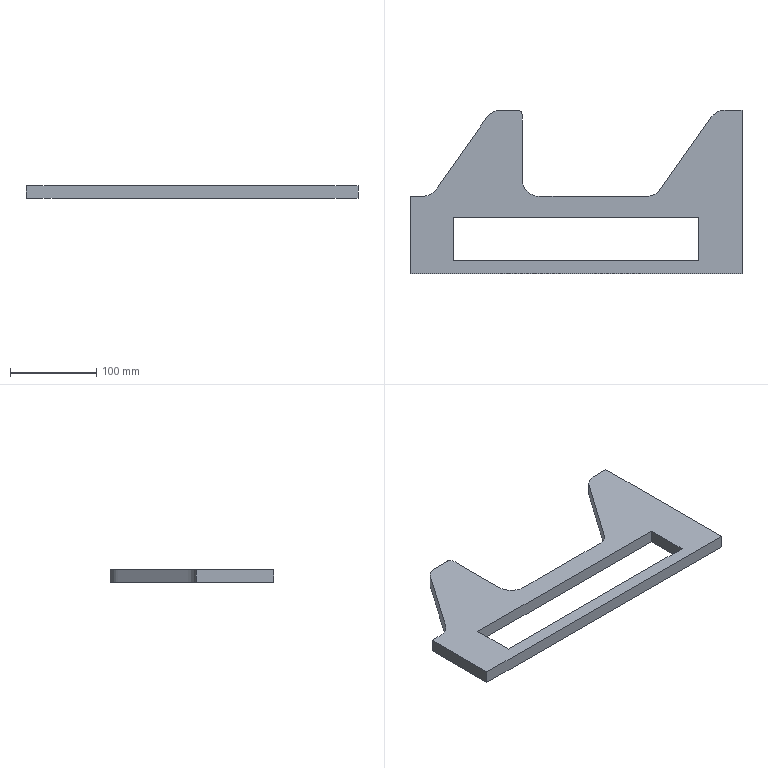Part | SolidWorks | features Extrusion 1 | 1 solid | 10 faces | box 385 x 190 x 15 mm | volume 496112 mm3 | plane 9 | spline 1
STEP:
#1=CARTESIAN_POINT('',(-385.,0.,15.));
#2=VERTEX_POINT('',#1);
#3=CARTESIAN_POINT('',(0.,0.,15.));
#4=VERTEX_POINT('',#3);
#5=CARTESIAN_POINT('',(-385.,0.,15.));
#6=DIRECTION('',(1.,0.,0.));
#7=VECTOR('',#6,1000.);
#8=LINE('',#5,#7);
#9=EDGE_CURVE('',#2,#4,#8,.T.);
#10=ORIENTED_EDGE('',*,*,#9,.T.);
#11=CARTESIAN_POINT('',(0.,190.,15.));
#12=VERTEX_POINT('',#11);
#13=CARTESIAN_POINT('',(0.,0.,15.));
#14=DIRECTION('',(0.,1.,0.));
#15=VECTOR('',#14,1000.);
#16=LINE('',#13,#15);
#17=EDGE_CURVE('',#4,#12,#16,.T.);
#18=ORIENTED_EDGE('',*,*,#17,.T.);
#19=CARTESIAN_POINT('',(-385.,90.,15.));
#20=VERTEX_POINT('',#19);
#21=CARTESIAN_POINT('',(0.,190.,15.));
#22=CARTESIAN_POINT('',(-6.53,190.,15.));
#23=CARTESIAN_POINT('',(-13.591,190.,15.));
#24=CARTESIAN_POINT('',(-21.185,190.,15.));
#25=CARTESIAN_POINT('',(-22.782,189.765,15.));
#26=CARTESIAN_POINT('',(-23.826,189.553,15.));
#27=CARTESIAN_POINT('',(-24.342,189.427,15.));
#28=CARTESIAN_POINT('',(-27.481,188.659,15.));
#29=CARTESIAN_POINT('',(-30.346,187.167,15.));
#30=CARTESIAN_POINT('',(-32.776,185.037,15.));
#31=CARTESIAN_POINT('',(-33.176,184.686,15.));
#32=CARTESIAN_POINT('',(-33.948,183.953,15.));
#33=CARTESIAN_POINT('',(-35.056,182.779,15.));
#34=CARTESIAN_POINT('',(-55.026,154.26,15.));
#35=CARTESIAN_POINT('',(-74.995,125.74,15.));
#36=CARTESIAN_POINT('',(-94.965,97.221,15.));
#37=CARTESIAN_POINT('',(-96.073,96.047,15.));
#38=CARTESIAN_POINT('',(-96.845,95.314,15.));
#39=CARTESIAN_POINT('',(-97.245,94.963,15.));
#40=CARTESIAN_POINT('',(-99.674,92.833,15.));
#41=CARTESIAN_POINT('',(-102.54,91.341,15.));
#42=CARTESIAN_POINT('',(-105.678,90.573,15.));
#43=CARTESIAN_POINT('',(-106.195,90.447,15.));
#44=CARTESIAN_POINT('',(-107.239,90.235,15.));
#45=CARTESIAN_POINT('',(-108.836,90.,15.));
#46=CARTESIAN_POINT('',(-151.423,90.,15.));
#47=CARTESIAN_POINT('',(-194.344,90.,15.));
#48=CARTESIAN_POINT('',(-237.601,90.,15.));
#49=CARTESIAN_POINT('',(-240.207,90.631,15.));
#50=CARTESIAN_POINT('',(-241.853,91.191,15.));
#51=CARTESIAN_POINT('',(-242.654,91.522,15.));
#52=CARTESIAN_POINT('',(-247.62,93.579,15.));
#53=CARTESIAN_POINT('',(-251.421,97.38,15.));
#54=CARTESIAN_POINT('',(-253.478,102.346,15.));
#55=CARTESIAN_POINT('',(-253.809,103.147,15.));
#56=CARTESIAN_POINT('',(-254.369,104.793,15.));
#57=CARTESIAN_POINT('',(-255.,107.399,15.));
#58=CARTESIAN_POINT('',(-255.,133.751,15.));
#59=CARTESIAN_POINT('',(-255.,160.201,15.));
#60=CARTESIAN_POINT('',(-255.,186.751,15.));
#61=CARTESIAN_POINT('',(-258.249,190.,15.));
#62=CARTESIAN_POINT('',(-266.328,190.,15.));
#63=CARTESIAN_POINT('',(-273.974,190.,15.));
#64=CARTESIAN_POINT('',(-281.185,190.,15.));
#65=CARTESIAN_POINT('',(-282.782,189.765,15.));
#66=CARTESIAN_POINT('',(-283.826,189.553,15.));
#67=CARTESIAN_POINT('',(-284.342,189.427,15.));
#68=CARTESIAN_POINT('',(-287.481,188.659,15.));
#69=CARTESIAN_POINT('',(-290.346,187.167,15.));
#70=CARTESIAN_POINT('',(-292.776,185.037,15.));
#71=CARTESIAN_POINT('',(-293.176,184.686,15.));
#72=CARTESIAN_POINT('',(-293.948,183.953,15.));
#73=CARTESIAN_POINT('',(-295.056,182.779,15.));
#74=CARTESIAN_POINT('',(-315.026,154.26,15.));
#75=CARTESIAN_POINT('',(-334.995,125.74,15.));
#76=CARTESIAN_POINT('',(-354.965,97.221,15.));
#77=CARTESIAN_POINT('',(-356.073,96.047,15.));
#78=CARTESIAN_POINT('',(-356.845,95.314,15.));
#79=CARTESIAN_POINT('',(-357.245,94.963,15.));
#80=CARTESIAN_POINT('',(-359.674,92.833,15.));
#81=CARTESIAN_POINT('',(-362.54,91.341,15.));
#82=CARTESIAN_POINT('',(-365.678,90.573,15.));
#83=CARTESIAN_POINT('',(-366.195,90.447,15.));
#84=CARTESIAN_POINT('',(-367.239,90.235,15.));
#85=CARTESIAN_POINT('',(-368.836,90.,15.));
#86=CARTESIAN_POINT('',(-374.756,90.,15.));
#87=CARTESIAN_POINT('',(-380.144,90.,15.));
#88=CARTESIAN_POINT('',(-385.,90.,15.));
#89=(BOUNDED_CURVE()B_SPLINE_CURVE(3,(#21,#22,#23,#24,#25,#26,#27,#28,#29,#30,#31,#32,#33,#34,#35,#36,#37,#38,#39,#40,#41,#42,#43,#44,#45,#46,#47,#48,#49,#50,#51,#52,#53,#54,#55,#56,#57,#58,#59,#60,#61,#62,#63,#64,#65,#66,#67,#68,#69,#70,#71,#72,#73,#74,#75,#76,#77,#78,#79,#80,#81,#82,#83,#84,#85,#86,#87,#88),.UNSPECIFIED.,.F.,.F.)B_SPLINE_CURVE_WITH_KNOTS((4,1,1,1,3,3,1,1,1,1,1,1,3,3,1,1,1,1,1,1,3,3,1,1,1,1,1,1,1,1,1,1,3,3,1,1,1,1,1,1,3,3,1,1,1,4),(0.,0.0344,0.0372,0.04,0.04281,0.0595,0.0623,0.06511,0.06791,0.2457,0.2485,0.2513,0.2541,0.2708,0.2736,0.2764,0.2792,0.498,0.5025,0.5071,0.5117,0.5386,0.5431,0.5477,0.5523,0.6819,0.687,0.6921,0.6972,0.7296,0.7324,0.7352,0.738,0.7547,0.7575,0.7603,0.7631,0.9409,0.9437,0.9465,0.9493,0.966,0.9688,0.9716,0.9744,1.),.UNSPECIFIED.)CURVE()GEOMETRIC_REPRESENTATION_ITEM()RATIONAL_B_SPLINE_CURVE((1.,1.,1.,1.,1.,1.,1.,0.9809,0.9809,1.,1.,1.,1.,1.,1.,1.,1.,1.,1.,0.9809,0.9809,1.,1.,1.,1.,1.,1.,1.,1.,1.,1.,0.9493,0.9493,1.,1.,1.,1.,1.,1.,1.,1.,1.,1.,1.,1.,1.,1.,0.9809,0.9809,1.,1.,1.,1.,1.,1.,1.,1.,1.,1.,0.9809,0.9809,1.,1.,1.,1.,1.,1.,1.))REPRESENTATION_ITEM(''));
#90=EDGE_CURVE('',#12,#20,#89,.T.);
#91=ORIENTED_EDGE('',*,*,#90,.T.);
#92=CARTESIAN_POINT('',(-385.,90.,15.));
#93=DIRECTION('',(0.,-1.,0.));
#94=VECTOR('',#93,1000.);
#95=LINE('',#92,#94);
#96=EDGE_CURVE('',#20,#2,#95,.T.);
#97=ORIENTED_EDGE('',*,*,#96,.T.);
#98=EDGE_LOOP('',(#10,#18,#91,#97));
#99=FACE_OUTER_BOUND('',#98,.T.);
#100=CARTESIAN_POINT('',(-335.,65.,15.));
#101=VERTEX_POINT('',#100);
#102=CARTESIAN_POINT('',(-335.,15.,15.));
#103=VERTEX_POINT('',#102);
#104=CARTESIAN_POINT('',(-335.,65.,15.));
#105=DIRECTION('',(0.,-1.,0.));
#106=VECTOR('',#105,1000.);
#107=LINE('',#104,#106);
#108=EDGE_CURVE('',#101,#103,#107,.T.);
#109=ORIENTED_EDGE('',*,*,#108,.F.);
#110=CARTESIAN_POINT('',(-50.,65.,15.));
#111=VERTEX_POINT('',#110);
#112=CARTESIAN_POINT('',(-335.,65.,15.));
#113=DIRECTION('',(-1.,0.,0.));
#114=VECTOR('',#113,1000.);
#115=LINE('',#112,#114);
#116=EDGE_CURVE('',#111,#101,#115,.T.);
#117=ORIENTED_EDGE('',*,*,#116,.F.);
#118=CARTESIAN_POINT('',(-50.,15.,15.));
#119=VERTEX_POINT('',#118);
#120=CARTESIAN_POINT('',(-50.,65.,15.));
#121=DIRECTION('',(0.,1.,0.));
#122=VECTOR('',#121,1000.);
#123=LINE('',#120,#122);
#124=EDGE_CURVE('',#119,#111,#123,.T.);
#125=ORIENTED_EDGE('',*,*,#124,.F.);
#126=CARTESIAN_POINT('',(-335.,15.,15.));
#127=DIRECTION('',(1.,0.,0.));
#128=VECTOR('',#127,1000.);
#129=LINE('',#126,#128);
#130=EDGE_CURVE('',#103,#119,#129,.T.);
#131=ORIENTED_EDGE('',*,*,#130,.F.);
#132=EDGE_LOOP('',(#109,#117,#125,#131));
#133=FACE_BOUND('',#132,.T.);
#134=CARTESIAN_POINT('',(-236.157,90.009,15.));
#135=DIRECTION('',(0.,0.,-1.));
#136=DIRECTION('',(-1.,0.,0.));
#137=AXIS2_PLACEMENT_3D('',#134,#135,#136);
#138=PLANE('',#137);
#139=ADVANCED_FACE('',(#99,#133),#138,.F.);
#140=CARTESIAN_POINT('',(-385.,0.,0.));
#141=VERTEX_POINT('',#140);
#142=CARTESIAN_POINT('',(0.,0.,0.));
#143=VERTEX_POINT('',#142);
#144=CARTESIAN_POINT('',(-385.,0.,0.));
#145=DIRECTION('',(1.,0.,0.));
#146=VECTOR('',#145,1000.);
#147=LINE('',#144,#146);
#148=EDGE_CURVE('',#141,#143,#147,.T.);
#149=ORIENTED_EDGE('',*,*,#148,.F.);
#150=CARTESIAN_POINT('',(-385.,90.,0.));
#151=VERTEX_POINT('',#150);
#152=CARTESIAN_POINT('',(-385.,90.,0.));
#153=DIRECTION('',(0.,-1.,0.));
#154=VECTOR('',#153,1000.);
#155=LINE('',#152,#154);
#156=EDGE_CURVE('',#151,#141,#155,.T.);
#157=ORIENTED_EDGE('',*,*,#156,.F.);
#158=CARTESIAN_POINT('',(0.,190.,0.));
#159=VERTEX_POINT('',#158);
#160=CARTESIAN_POINT('',(0.,190.,0.));
#161=CARTESIAN_POINT('',(-6.53,190.,0.));
#162=CARTESIAN_POINT('',(-13.591,190.,0.));
#163=CARTESIAN_POINT('',(-21.185,190.,0.));
#164=CARTESIAN_POINT('',(-22.782,189.765,0.));
#165=CARTESIAN_POINT('',(-23.826,189.553,0.));
#166=CARTESIAN_POINT('',(-24.342,189.427,0.));
#167=CARTESIAN_POINT('',(-27.481,188.659,0.));
#168=CARTESIAN_POINT('',(-30.346,187.167,0.));
#169=CARTESIAN_POINT('',(-32.776,185.037,0.));
#170=CARTESIAN_POINT('',(-33.176,184.686,0.));
#171=CARTESIAN_POINT('',(-33.948,183.953,0.));
#172=CARTESIAN_POINT('',(-35.056,182.779,0.));
#173=CARTESIAN_POINT('',(-55.026,154.26,0.));
#174=CARTESIAN_POINT('',(-74.995,125.74,0.));
#175=CARTESIAN_POINT('',(-94.965,97.221,0.));
#176=CARTESIAN_POINT('',(-96.073,96.047,0.));
#177=CARTESIAN_POINT('',(-96.845,95.314,0.));
#178=CARTESIAN_POINT('',(-97.245,94.963,0.));
#179=CARTESIAN_POINT('',(-99.674,92.833,0.));
#180=CARTESIAN_POINT('',(-102.54,91.341,0.));
#181=CARTESIAN_POINT('',(-105.678,90.573,0.));
#182=CARTESIAN_POINT('',(-106.195,90.447,0.));
#183=CARTESIAN_POINT('',(-107.239,90.235,0.));
#184=CARTESIAN_POINT('',(-108.836,90.,0.));
#185=CARTESIAN_POINT('',(-151.423,90.,0.));
#186=CARTESIAN_POINT('',(-194.344,90.,0.));
#187=CARTESIAN_POINT('',(-237.601,90.,0.));
#188=CARTESIAN_POINT('',(-240.207,90.631,0.));
#189=CARTESIAN_POINT('',(-241.853,91.191,0.));
#190=CARTESIAN_POINT('',(-242.654,91.522,0.));
#191=CARTESIAN_POINT('',(-247.62,93.579,0.));
#192=CARTESIAN_POINT('',(-251.421,97.38,0.));
#193=CARTESIAN_POINT('',(-253.478,102.346,0.));
#194=CARTESIAN_POINT('',(-253.809,103.147,0.));
#195=CARTESIAN_POINT('',(-254.369,104.793,0.));
#196=CARTESIAN_POINT('',(-255.,107.399,0.));
#197=CARTESIAN_POINT('',(-255.,133.751,0.));
#198=CARTESIAN_POINT('',(-255.,160.201,0.));
#199=CARTESIAN_POINT('',(-255.,186.751,0.));
#200=CARTESIAN_POINT('',(-258.249,190.,0.));
#201=CARTESIAN_POINT('',(-266.328,190.,0.));
#202=CARTESIAN_POINT('',(-273.974,190.,0.));
#203=CARTESIAN_POINT('',(-281.185,190.,0.));
#204=CARTESIAN_POINT('',(-282.782,189.765,0.));
#205=CARTESIAN_POINT('',(-283.826,189.553,0.));
#206=CARTESIAN_POINT('',(-284.342,189.427,0.));
#207=CARTESIAN_POINT('',(-287.481,188.659,0.));
#208=CARTESIAN_POINT('',(-290.346,187.167,0.));
#209=CARTESIAN_POINT('',(-292.776,185.037,0.));
#210=CARTESIAN_POINT('',(-293.176,184.686,0.));
#211=CARTESIAN_POINT('',(-293.948,183.953,0.));
#212=CARTESIAN_POINT('',(-295.056,182.779,0.));
#213=CARTESIAN_POINT('',(-315.026,154.26,0.));
#214=CARTESIAN_POINT('',(-334.995,125.74,0.));
#215=CARTESIAN_POINT('',(-354.965,97.221,0.));
#216=CARTESIAN_POINT('',(-356.073,96.047,0.));
#217=CARTESIAN_POINT('',(-356.845,95.314,0.));
#218=CARTESIAN_POINT('',(-357.245,94.963,0.));
#219=CARTESIAN_POINT('',(-359.674,92.833,0.));
#220=CARTESIAN_POINT('',(-362.54,91.341,0.));
#221=CARTESIAN_POINT('',(-365.678,90.573,0.));
#222=CARTESIAN_POINT('',(-366.195,90.447,0.));
#223=CARTESIAN_POINT('',(-367.239,90.235,0.));
#224=CARTESIAN_POINT('',(-368.836,90.,0.));
#225=CARTESIAN_POINT('',(-374.756,90.,0.));
#226=CARTESIAN_POINT('',(-380.144,90.,0.));
#227=CARTESIAN_POINT('',(-385.,90.,0.));
#228=(BOUNDED_CURVE()B_SPLINE_CURVE(3,(#160,#161,#162,#163,#164,#165,#166,#167,#168,#169,#170,#171,#172,#173,#174,#175,#176,#177,#178,#179,#180,#181,#182,#183,#184,#185,#186,#187,#188,#189,#190,#191,#192,#193,#194,#195,#196,#197,#198,#199,#200,#201,#202,#203,#204,#205,#206,#207,#208,#209,#210,#211,#212,#213,#214,#215,#216,#217,#218,#219,#220,#221,#222,#223,#224,#225,#226,#227),.UNSPECIFIED.,.F.,.T.)B_SPLINE_CURVE_WITH_KNOTS((4,1,1,1,3,3,1,1,1,1,1,1,3,3,1,1,1,1,1,1,3,3,1,1,1,1,1,1,1,1,1,1,3,3,1,1,1,1,1,1,3,3,1,1,1,4),(0.,0.0344,0.0372,0.04,0.04281,0.0595,0.0623,0.06511,0.06791,0.2457,0.2485,0.2513,0.2541,0.2708,0.2736,0.2764,0.2792,0.498,0.5025,0.5071,0.5117,0.5386,0.5431,0.5477,0.5523,0.6819,0.687,0.6921,0.6972,0.7296,0.7324,0.7352,0.738,0.7547,0.7575,0.7603,0.7631,0.9409,0.9437,0.9465,0.9493,0.966,0.9688,0.9716,0.9744,1.),.UNSPECIFIED.)CURVE()GEOMETRIC_REPRESENTATION_ITEM()RATIONAL_B_SPLINE_CURVE((1.,1.,1.,1.,1.,1.,1.,0.9809,0.9809,1.,1.,1.,1.,1.,1.,1.,1.,1.,1.,0.9809,0.9809,1.,1.,1.,1.,1.,1.,1.,1.,1.,1.,0.9493,0.9493,1.,1.,1.,1.,1.,1.,1.,1.,1.,1.,1.,1.,1.,1.,0.9809,0.9809,1.,1.,1.,1.,1.,1.,1.,1.,1.,1.,0.9809,0.9809,1.,1.,1.,1.,1.,1.,1.))REPRESENTATION_ITEM(''));
#229=EDGE_CURVE('',#159,#151,#228,.T.);
#230=ORIENTED_EDGE('',*,*,#229,.F.);
#231=CARTESIAN_POINT('',(0.,0.,0.));
#232=DIRECTION('',(0.,1.,0.));
#233=VECTOR('',#232,1000.);
#234=LINE('',#231,#233);
#235=EDGE_CURVE('',#143,#159,#234,.T.);
#236=ORIENTED_EDGE('',*,*,#235,.F.);
#237=EDGE_LOOP('',(#149,#157,#230,#236));
#238=FACE_OUTER_BOUND('',#237,.T.);
#239=CARTESIAN_POINT('',(-50.,65.,0.));
#240=VERTEX_POINT('',#239);
#241=CARTESIAN_POINT('',(-335.,65.,0.));
#242=VERTEX_POINT('',#241);
#243=CARTESIAN_POINT('',(-335.,65.,0.));
#244=DIRECTION('',(-1.,0.,0.));
#245=VECTOR('',#244,1000.);
#246=LINE('',#243,#245);
#247=EDGE_CURVE('',#240,#242,#246,.T.);
#248=ORIENTED_EDGE('',*,*,#247,.T.);
#249=CARTESIAN_POINT('',(-335.,15.,0.));
#250=VERTEX_POINT('',#249);
#251=CARTESIAN_POINT('',(-335.,65.,0.));
#252=DIRECTION('',(0.,-1.,0.));
#253=VECTOR('',#252,1000.);
#254=LINE('',#251,#253);
#255=EDGE_CURVE('',#242,#250,#254,.T.);
#256=ORIENTED_EDGE('',*,*,#255,.T.);
#257=CARTESIAN_POINT('',(-50.,15.,0.));
#258=VERTEX_POINT('',#257);
#259=CARTESIAN_POINT('',(-335.,15.,0.));
#260=DIRECTION('',(1.,0.,0.));
#261=VECTOR('',#260,1000.);
#262=LINE('',#259,#261);
#263=EDGE_CURVE('',#250,#258,#262,.T.);
#264=ORIENTED_EDGE('',*,*,#263,.T.);
#265=CARTESIAN_POINT('',(-50.,65.,0.));
#266=DIRECTION('',(0.,1.,0.));
#267=VECTOR('',#266,1000.);
#268=LINE('',#265,#267);
#269=EDGE_CURVE('',#258,#240,#268,.T.);
#270=ORIENTED_EDGE('',*,*,#269,.T.);
#271=EDGE_LOOP('',(#248,#256,#264,#270));
#272=FACE_BOUND('',#271,.T.);
#273=CARTESIAN_POINT('',(-236.157,90.009,0.));
#274=DIRECTION('',(0.,0.,-1.));
#275=DIRECTION('',(-1.,0.,0.));
#276=AXIS2_PLACEMENT_3D('',#273,#274,#275);
#277=PLANE('',#276);
#278=ADVANCED_FACE('',(#238,#272),#277,.T.);
#279=ORIENTED_EDGE('',*,*,#148,.T.);
#280=CARTESIAN_POINT('',(0.,0.,15.));
#281=DIRECTION('',(0.,0.,-1.));
#282=VECTOR('',#281,1000.);
#283=LINE('',#280,#282);
#284=EDGE_CURVE('',#4,#143,#283,.T.);
#285=ORIENTED_EDGE('',*,*,#284,.F.);
#286=ORIENTED_EDGE('',*,*,#9,.F.);
#287=CARTESIAN_POINT('',(-385.,0.,15.));
#288=DIRECTION('',(0.,0.,-1.));
#289=VECTOR('',#288,1000.);
#290=LINE('',#287,#289);
#291=EDGE_CURVE('',#2,#141,#290,.T.);
#292=ORIENTED_EDGE('',*,*,#291,.T.);
#293=EDGE_LOOP('',(#279,#285,#286,#292));
#294=FACE_OUTER_BOUND('',#293,.T.);
#295=CARTESIAN_POINT('',(-385.,0.,15.));
#296=DIRECTION('',(0.,1.,0.));
#297=DIRECTION('',(0.,0.,1.));
#298=AXIS2_PLACEMENT_3D('',#295,#296,#297);
#299=PLANE('',#298);
#300=ADVANCED_FACE('',(#294),#299,.F.);
#301=ORIENTED_EDGE('',*,*,#235,.T.);
#302=CARTESIAN_POINT('',(0.,190.,15.));
#303=DIRECTION('',(0.,0.,-1.));
#304=VECTOR('',#303,1000.);
#305=LINE('',#302,#304);
#306=EDGE_CURVE('',#12,#159,#305,.T.);
#307=ORIENTED_EDGE('',*,*,#306,.F.);
#308=ORIENTED_EDGE('',*,*,#17,.F.);
#309=ORIENTED_EDGE('',*,*,#284,.T.);
#310=EDGE_LOOP('',(#301,#307,#308,#309));
#311=FACE_OUTER_BOUND('',#310,.T.);
#312=CARTESIAN_POINT('',(0.,0.,15.));
#313=DIRECTION('',(-1.,0.,0.));
#314=DIRECTION('',(0.,0.,1.));
#315=AXIS2_PLACEMENT_3D('',#312,#313,#314);
#316=PLANE('',#315);
#317=ADVANCED_FACE('',(#311),#316,.F.);
#318=ORIENTED_EDGE('',*,*,#229,.T.);
#319=CARTESIAN_POINT('',(-385.,90.,15.));
#320=DIRECTION('',(0.,0.,-1.));
#321=VECTOR('',#320,1000.);
#322=LINE('',#319,#321);
#323=EDGE_CURVE('',#20,#151,#322,.T.);
#324=ORIENTED_EDGE('',*,*,#323,.F.);
#325=ORIENTED_EDGE('',*,*,#90,.F.);
#326=ORIENTED_EDGE('',*,*,#306,.T.);
#327=EDGE_LOOP('',(#318,#324,#325,#326));
#328=FACE_OUTER_BOUND('',#327,.T.);
#329=CARTESIAN_POINT('',(0.,190.,15.));
#330=CARTESIAN_POINT('',(0.,190.,0.));
#331=CARTESIAN_POINT('',(-6.53,190.,15.));
#332=CARTESIAN_POINT('',(-6.53,190.,0.));
#333=CARTESIAN_POINT('',(-13.591,190.,15.));
#334=CARTESIAN_POINT('',(-13.591,190.,0.));
#335=CARTESIAN_POINT('',(-21.185,190.,15.));
#336=CARTESIAN_POINT('',(-21.185,190.,0.));
#337=CARTESIAN_POINT('',(-22.782,189.765,15.));
#338=CARTESIAN_POINT('',(-22.782,189.765,0.));
#339=CARTESIAN_POINT('',(-23.826,189.553,15.));
#340=CARTESIAN_POINT('',(-23.826,189.553,0.));
#341=CARTESIAN_POINT('',(-24.342,189.427,15.));
#342=CARTESIAN_POINT('',(-24.342,189.427,0.));
#343=CARTESIAN_POINT('',(-27.481,188.659,15.));
#344=CARTESIAN_POINT('',(-27.481,188.659,0.));
#345=CARTESIAN_POINT('',(-30.346,187.167,15.));
#346=CARTESIAN_POINT('',(-30.346,187.167,0.));
#347=CARTESIAN_POINT('',(-32.776,185.037,15.));
#348=CARTESIAN_POINT('',(-32.776,185.037,0.));
#349=CARTESIAN_POINT('',(-33.176,184.686,15.));
#350=CARTESIAN_POINT('',(-33.176,184.686,0.));
#351=CARTESIAN_POINT('',(-33.948,183.953,15.));
#352=CARTESIAN_POINT('',(-33.948,183.953,0.));
#353=CARTESIAN_POINT('',(-35.056,182.779,15.));
#354=CARTESIAN_POINT('',(-35.056,182.779,0.));
#355=CARTESIAN_POINT('',(-55.026,154.26,15.));
#356=CARTESIAN_POINT('',(-55.026,154.26,0.));
#357=CARTESIAN_POINT('',(-74.995,125.74,15.));
#358=CARTESIAN_POINT('',(-74.995,125.74,0.));
#359=CARTESIAN_POINT('',(-94.965,97.221,15.));
#360=CARTESIAN_POINT('',(-94.965,97.221,0.));
#361=CARTESIAN_POINT('',(-96.073,96.047,15.));
#362=CARTESIAN_POINT('',(-96.073,96.047,0.));
#363=CARTESIAN_POINT('',(-96.845,95.314,15.));
#364=CARTESIAN_POINT('',(-96.845,95.314,0.));
#365=CARTESIAN_POINT('',(-97.245,94.963,15.));
#366=CARTESIAN_POINT('',(-97.245,94.963,0.));
#367=CARTESIAN_POINT('',(-99.674,92.833,15.));
#368=CARTESIAN_POINT('',(-99.674,92.833,0.));
#369=CARTESIAN_POINT('',(-102.54,91.341,15.));
#370=CARTESIAN_POINT('',(-102.54,91.341,0.));
#371=CARTESIAN_POINT('',(-105.678,90.573,15.));
#372=CARTESIAN_POINT('',(-105.678,90.573,0.));
#373=CARTESIAN_POINT('',(-106.195,90.447,15.));
#374=CARTESIAN_POINT('',(-106.195,90.447,0.));
#375=CARTESIAN_POINT('',(-107.239,90.235,15.));
#376=CARTESIAN_POINT('',(-107.239,90.235,0.));
#377=CARTESIAN_POINT('',(-108.836,90.,15.));
#378=CARTESIAN_POINT('',(-108.836,90.,0.));
#379=CARTESIAN_POINT('',(-151.423,90.,15.));
#380=CARTESIAN_POINT('',(-151.423,90.,0.));
#381=CARTESIAN_POINT('',(-194.344,90.,15.));
#382=CARTESIAN_POINT('',(-194.344,90.,0.));
#383=CARTESIAN_POINT('',(-237.601,90.,15.));
#384=CARTESIAN_POINT('',(-237.601,90.,0.));
#385=CARTESIAN_POINT('',(-240.207,90.631,15.));
#386=CARTESIAN_POINT('',(-240.207,90.631,0.));
#387=CARTESIAN_POINT('',(-241.853,91.191,15.));
#388=CARTESIAN_POINT('',(-241.853,91.191,0.));
#389=CARTESIAN_POINT('',(-242.654,91.522,15.));
#390=CARTESIAN_POINT('',(-242.654,91.522,0.));
#391=CARTESIAN_POINT('',(-247.62,93.579,15.));
#392=CARTESIAN_POINT('',(-247.62,93.579,0.));
#393=CARTESIAN_POINT('',(-251.421,97.38,15.));
#394=CARTESIAN_POINT('',(-251.421,97.38,0.));
#395=CARTESIAN_POINT('',(-253.478,102.346,15.));
#396=CARTESIAN_POINT('',(-253.478,102.346,0.));
#397=CARTESIAN_POINT('',(-253.809,103.147,15.));
#398=CARTESIAN_POINT('',(-253.809,103.147,0.));
#399=CARTESIAN_POINT('',(-254.369,104.793,15.));
#400=CARTESIAN_POINT('',(-254.369,104.793,0.));
#401=CARTESIAN_POINT('',(-255.,107.399,15.));
#402=CARTESIAN_POINT('',(-255.,107.399,0.));
#403=CARTESIAN_POINT('',(-255.,133.751,15.));
#404=CARTESIAN_POINT('',(-255.,133.751,0.));
#405=CARTESIAN_POINT('',(-255.,160.201,15.));
#406=CARTESIAN_POINT('',(-255.,160.201,0.));
#407=CARTESIAN_POINT('',(-255.,186.751,15.));
#408=CARTESIAN_POINT('',(-255.,186.751,0.));
#409=CARTESIAN_POINT('',(-258.249,190.,15.));
#410=CARTESIAN_POINT('',(-258.249,190.,0.));
#411=CARTESIAN_POINT('',(-266.328,190.,15.));
#412=CARTESIAN_POINT('',(-266.328,190.,0.));
#413=CARTESIAN_POINT('',(-273.974,190.,15.));
#414=CARTESIAN_POINT('',(-273.974,190.,0.));
#415=CARTESIAN_POINT('',(-281.185,190.,15.));
#416=CARTESIAN_POINT('',(-281.185,190.,0.));
#417=CARTESIAN_POINT('',(-282.782,189.765,15.));
#418=CARTESIAN_POINT('',(-282.782,189.765,0.));
#419=CARTESIAN_POINT('',(-283.826,189.553,15.));
#420=CARTESIAN_POINT('',(-283.826,189.553,0.));
#421=CARTESIAN_POINT('',(-284.342,189.427,15.));
#422=CARTESIAN_POINT('',(-284.342,189.427,0.));
#423=CARTESIAN_POINT('',(-287.481,188.659,15.));
#424=CARTESIAN_POINT('',(-287.481,188.659,0.));
#425=CARTESIAN_POINT('',(-290.346,187.167,15.));
#426=CARTESIAN_POINT('',(-290.346,187.167,0.));
#427=CARTESIAN_POINT('',(-292.776,185.037,15.));
#428=CARTESIAN_POINT('',(-292.776,185.037,0.));
#429=CARTESIAN_POINT('',(-293.176,184.686,15.));
#430=CARTESIAN_POINT('',(-293.176,184.686,0.));
#431=CARTESIAN_POINT('',(-293.948,183.953,15.));
#432=CARTESIAN_POINT('',(-293.948,183.953,0.));
#433=CARTESIAN_POINT('',(-295.056,182.779,15.));
#434=CARTESIAN_POINT('',(-295.056,182.779,0.));
#435=CARTESIAN_POINT('',(-315.026,154.26,15.));
#436=CARTESIAN_POINT('',(-315.026,154.26,0.));
#437=CARTESIAN_POINT('',(-334.995,125.74,15.));
#438=CARTESIAN_POINT('',(-334.995,125.74,0.));
#439=CARTESIAN_POINT('',(-354.965,97.221,15.));
#440=CARTESIAN_POINT('',(-354.965,97.221,0.));
#441=CARTESIAN_POINT('',(-356.073,96.047,15.));
#442=CARTESIAN_POINT('',(-356.073,96.047,0.));
#443=CARTESIAN_POINT('',(-356.845,95.314,15.));
#444=CARTESIAN_POINT('',(-356.845,95.314,0.));
#445=CARTESIAN_POINT('',(-357.245,94.963,15.));
#446=CARTESIAN_POINT('',(-357.245,94.963,0.));
#447=CARTESIAN_POINT('',(-359.674,92.833,15.));
#448=CARTESIAN_POINT('',(-359.674,92.833,0.));
#449=CARTESIAN_POINT('',(-362.54,91.341,15.));
#450=CARTESIAN_POINT('',(-362.54,91.341,0.));
#451=CARTESIAN_POINT('',(-365.678,90.573,15.));
#452=CARTESIAN_POINT('',(-365.678,90.573,0.));
#453=CARTESIAN_POINT('',(-366.195,90.447,15.));
#454=CARTESIAN_POINT('',(-366.195,90.447,0.));
#455=CARTESIAN_POINT('',(-367.239,90.235,15.));
#456=CARTESIAN_POINT('',(-367.239,90.235,0.));
#457=CARTESIAN_POINT('',(-368.836,90.,15.));
#458=CARTESIAN_POINT('',(-368.836,90.,0.));
#459=CARTESIAN_POINT('',(-374.756,90.,15.));
#460=CARTESIAN_POINT('',(-374.756,90.,0.));
#461=CARTESIAN_POINT('',(-380.144,90.,15.));
#462=CARTESIAN_POINT('',(-380.144,90.,0.));
#463=CARTESIAN_POINT('',(-385.,90.,15.));
#464=CARTESIAN_POINT('',(-385.,90.,0.));
#465=(BOUNDED_SURFACE()B_SPLINE_SURFACE(3,1,((#329,#330),(#331,#332),(#333,#334),(#335,#336),(#337,#338),(#339,#340),(#341,#342),(#343,#344),(#345,#346),(#347,#348),(#349,#350),(#351,#352),(#353,#354),(#355,#356),(#357,#358),(#359,#360),(#361,#362),(#363,#364),(#365,#366),(#367,#368),(#369,#370),(#371,#372),(#373,#374),(#375,#376),(#377,#378),(#379,#380),(#381,#382),(#383,#384),(#385,#386),(#387,#388),(#389,#390),(#391,#392),(#393,#394),(#395,#396),(#397,#398),(#399,#400),(#401,#402),(#403,#404),(#405,#406),(#407,#408),(#409,#410),(#411,#412),(#413,#414),(#415,#416),(#417,#418),(#419,#420),(#421,#422),(#423,#424),(#425,#426),(#427,#428),(#429,#430),(#431,#432),(#433,#434),(#435,#436),(#437,#438),(#439,#440),(#441,#442),(#443,#444),(#445,#446),(#447,#448),(#449,#450),(#451,#452),(#453,#454),(#455,#456),(#457,#458),(#459,#460),(#461,#462),(#463,#464)),.UNSPECIFIED.,.F.,.F.,.F.)B_SPLINE_SURFACE_WITH_KNOTS((4,1,1,1,3,3,1,1,1,1,1,1,3,3,1,1,1,1,1,1,3,3,1,1,1,1,1,1,1,1,1,1,3,3,1,1,1,1,1,1,3,3,1,1,1,4),(2,2),(0.,0.0344,0.0372,0.04,0.04281,0.0595,0.0623,0.06511,0.06791,0.2457,0.2485,0.2513,0.2541,0.2708,0.2736,0.2764,0.2792,0.498,0.5025,0.5071,0.5117,0.5386,0.5431,0.5477,0.5523,0.6819,0.687,0.6921,0.6972,0.7296,0.7324,0.7352,0.738,0.7547,0.7575,0.7603,0.7631,0.9409,0.9437,0.9465,0.9493,0.966,0.9688,0.9716,0.9744,1.),(0.,1.),.UNSPECIFIED.)GEOMETRIC_REPRESENTATION_ITEM()RATIONAL_B_SPLINE_SURFACE(((1.,1.),(1.,1.),(1.,1.),(1.,1.),(1.,1.),(1.,1.),(1.,1.),(0.9809,0.9809),(0.9809,0.9809),(1.,1.),(1.,1.),(1.,1.),(1.,1.),(1.,1.),(1.,1.),(1.,1.),(1.,1.),(1.,1.),(1.,1.),(0.9809,0.9809),(0.9809,0.9809),(1.,1.),(1.,1.),(1.,1.),(1.,1.),(1.,1.),(1.,1.),(1.,1.),(1.,1.),(1.,1.),(1.,1.),(0.9493,0.9493),(0.9493,0.9493),(1.,1.),(1.,1.),(1.,1.),(1.,1.),(1.,1.),(1.,1.),(1.,1.),(1.,1.),(1.,1.),(1.,1.),(1.,1.),(1.,1.),(1.,1.),(1.,1.),(0.9809,0.9809),(0.9809,0.9809),(1.,1.),(1.,1.),(1.,1.),(1.,1.),(1.,1.),(1.,1.),(1.,1.),(1.,1.),(1.,1.),(1.,1.),(0.9809,0.9809),(0.9809,0.9809),(1.,1.),(1.,1.),(1.,1.),(1.,1.),(1.,1.),(1.,1.),(1.,1.)))REPRESENTATION_ITEM('')SURFACE());
#466=ADVANCED_FACE('',(#328),#465,.F.);
#467=ORIENTED_EDGE('',*,*,#156,.T.);
#468=ORIENTED_EDGE('',*,*,#291,.F.);
#469=ORIENTED_EDGE('',*,*,#96,.F.);
#470=ORIENTED_EDGE('',*,*,#323,.T.);
#471=EDGE_LOOP('',(#467,#468,#469,#470));
#472=FACE_OUTER_BOUND('',#471,.T.);
#473=CARTESIAN_POINT('',(-385.,90.,15.));
#474=DIRECTION('',(1.,0.,0.));
#475=DIRECTION('',(0.,0.,-1.));
#476=AXIS2_PLACEMENT_3D('',#473,#474,#475);
#477=PLANE('',#476);
#478=ADVANCED_FACE('',(#472),#477,.F.);
#479=ORIENTED_EDGE('',*,*,#255,.F.);
#480=CARTESIAN_POINT('',(-335.,65.,15.));
#481=DIRECTION('',(0.,0.,-1.));
#482=VECTOR('',#481,1000.);
#483=LINE('',#480,#482);
#484=EDGE_CURVE('',#101,#242,#483,.T.);
#485=ORIENTED_EDGE('',*,*,#484,.F.);
#486=ORIENTED_EDGE('',*,*,#108,.T.);
#487=CARTESIAN_POINT('',(-335.,15.,15.));
#488=DIRECTION('',(0.,0.,-1.));
#489=VECTOR('',#488,1000.);
#490=LINE('',#487,#489);
#491=EDGE_CURVE('',#103,#250,#490,.T.);
#492=ORIENTED_EDGE('',*,*,#491,.T.);
#493=EDGE_LOOP('',(#479,#485,#486,#492));
#494=FACE_OUTER_BOUND('',#493,.T.);
#495=CARTESIAN_POINT('',(-335.,65.,15.));
#496=DIRECTION('',(1.,0.,0.));
#497=DIRECTION('',(0.,0.,-1.));
#498=AXIS2_PLACEMENT_3D('',#495,#496,#497);
#499=PLANE('',#498);
#500=ADVANCED_FACE('',(#494),#499,.T.);
#501=ORIENTED_EDGE('',*,*,#263,.F.);
#502=ORIENTED_EDGE('',*,*,#491,.F.);
#503=ORIENTED_EDGE('',*,*,#130,.T.);
#504=CARTESIAN_POINT('',(-50.,15.,15.));
#505=DIRECTION('',(0.,0.,-1.));
#506=VECTOR('',#505,1000.);
#507=LINE('',#504,#506);
#508=EDGE_CURVE('',#119,#258,#507,.T.);
#509=ORIENTED_EDGE('',*,*,#508,.T.);
#510=EDGE_LOOP('',(#501,#502,#503,#509));
#511=FACE_OUTER_BOUND('',#510,.T.);
#512=CARTESIAN_POINT('',(-335.,15.,15.));
#513=DIRECTION('',(0.,1.,0.));
#514=DIRECTION('',(0.,0.,1.));
#515=AXIS2_PLACEMENT_3D('',#512,#513,#514);
#516=PLANE('',#515);
#517=ADVANCED_FACE('',(#511),#516,.T.);
#518=ORIENTED_EDGE('',*,*,#269,.F.);
#519=ORIENTED_EDGE('',*,*,#508,.F.);
#520=ORIENTED_EDGE('',*,*,#124,.T.);
#521=CARTESIAN_POINT('',(-50.,65.,15.));
#522=DIRECTION('',(0.,0.,-1.));
#523=VECTOR('',#522,1000.);
#524=LINE('',#521,#523);
#525=EDGE_CURVE('',#111,#240,#524,.T.);
#526=ORIENTED_EDGE('',*,*,#525,.T.);
#527=EDGE_LOOP('',(#518,#519,#520,#526));
#528=FACE_OUTER_BOUND('',#527,.T.);
#529=CARTESIAN_POINT('',(-50.,65.,15.));
#530=DIRECTION('',(-1.,0.,0.));
#531=DIRECTION('',(0.,0.,1.));
#532=AXIS2_PLACEMENT_3D('',#529,#530,#531);
#533=PLANE('',#532);
#534=ADVANCED_FACE('',(#528),#533,.T.);
#535=ORIENTED_EDGE('',*,*,#247,.F.);
#536=ORIENTED_EDGE('',*,*,#525,.F.);
#537=ORIENTED_EDGE('',*,*,#116,.T.);
#538=ORIENTED_EDGE('',*,*,#484,.T.);
#539=EDGE_LOOP('',(#535,#536,#537,#538));
#540=FACE_OUTER_BOUND('',#539,.T.);
#541=CARTESIAN_POINT('',(-335.,65.,15.));
#542=DIRECTION('',(0.,-1.,0.));
#543=DIRECTION('',(0.,0.,-1.));
#544=AXIS2_PLACEMENT_3D('',#541,#542,#543);
#545=PLANE('',#544);
#546=ADVANCED_FACE('',(#540),#545,.T.);
#547=CLOSED_SHELL('',(#139,#278,#300,#317,#466,#478,#500,#517,#534,#546));
#548=MANIFOLD_SOLID_BREP('',#547);
#549=CARTESIAN_POINT('',(0.,0.,0.));
#550=DIRECTION('',(0.,0.,1.));
#551=DIRECTION('',(1.,0.,0.));
#552=AXIS2_PLACEMENT_3D('',#549,#550,#551);
#553=(LENGTH_UNIT()NAMED_UNIT(*)SI_UNIT(.MILLI.,.METRE.));
#554=UNCERTAINTY_MEASURE_WITH_UNIT(LENGTH_MEASURE(0.00001),#553,'','');
#555=(NAMED_UNIT(*)PLANE_ANGLE_UNIT()SI_UNIT($,.RADIAN.));
#556=(NAMED_UNIT(*)SI_UNIT($,.STERADIAN.)SOLID_ANGLE_UNIT());
#557=(GEOMETRIC_REPRESENTATION_CONTEXT(3)GLOBAL_UNCERTAINTY_ASSIGNED_CONTEXT((#554))GLOBAL_UNIT_ASSIGNED_CONTEXT((#553,#555,#556))REPRESENTATION_CONTEXT('',''));
#558=ADVANCED_BREP_SHAPE_REPRESENTATION('',(#548,#552),#557);